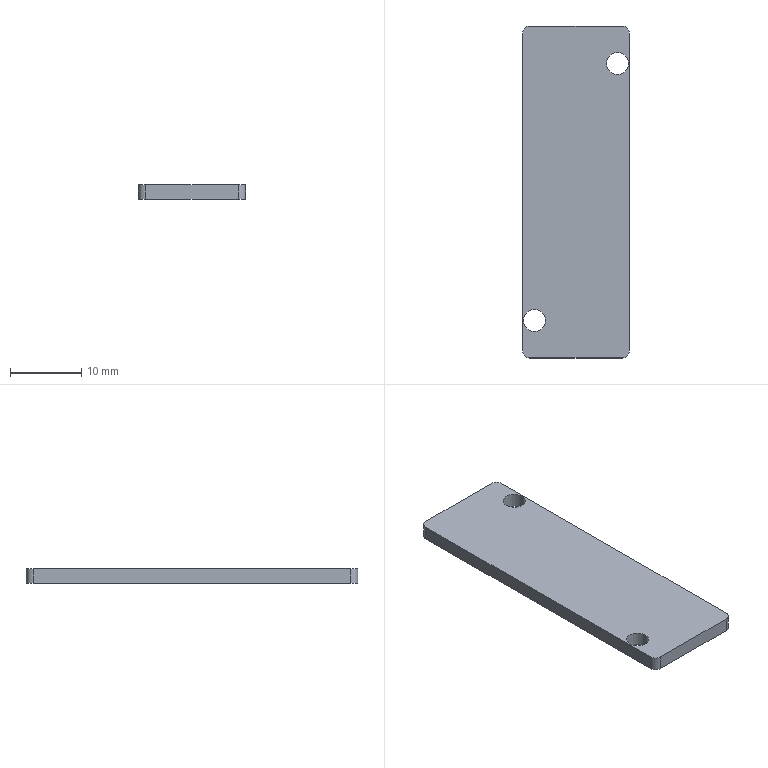Part | STEP file | Blind plate 7V100M | 1 solid | 14 faces | box 15 x 46.5 x 2 mm | volume 1363 mm3 | cylinder 8 | plane 6 | commonest cylinder face diameters 2 x4 3.1 x4
STEP:
#1=CARTESIAN_POINT('',(0.,0.,0.));
#2=DIRECTION('',(0.,0.,1.));
#3=DIRECTION('',(1.,0.,0.));
#4=AXIS2_PLACEMENT_3D('',#1,#2,#3);
#5=CARTESIAN_POINT('',(7.35,18.,0.));
#6=VERTEX_POINT('',#5);
#7=CARTESIAN_POINT('',(7.35,18.,2.));
#8=VERTEX_POINT('',#7);
#9=CARTESIAN_POINT('',(7.35,18.,0.));
#10=DIRECTION('',(0.,0.,1.));
#11=VECTOR('',#10,1.);
#12=LINE('',#9,#11);
#13=CARTESIAN_POINT('',(5.8,18.,0.));
#14=DIRECTION('',(0.,0.,1.));
#15=DIRECTION('',(1.,0.,0.));
#16=AXIS2_PLACEMENT_3D('',#13,#14,#15);
#17=CYLINDRICAL_SURFACE('',#16,1.55);
#18=CARTESIAN_POINT('',(6.283,0.));
#19=DIRECTION('',(0.,1.));
#20=VECTOR('',#19,1.);
#21=LINE('',#18,#20);
#22=(GEOMETRIC_REPRESENTATION_CONTEXT(2)PARAMETRIC_REPRESENTATION_CONTEXT()REPRESENTATION_CONTEXT('',''));
#23=DEFINITIONAL_REPRESENTATION('',(#21),#22);
#24=PCURVE('',#17,#23);
#25=CARTESIAN_POINT('',(5.8,18.,0.));
#26=DIRECTION('',(0.,0.,1.));
#27=DIRECTION('',(1.,0.,0.));
#28=AXIS2_PLACEMENT_3D('',#25,#26,#27);
#29=CYLINDRICAL_SURFACE('',#28,1.55);
#30=CARTESIAN_POINT('',(0.,0.));
#31=DIRECTION('',(0.,1.));
#32=VECTOR('',#31,1.);
#33=LINE('',#30,#32);
#34=(GEOMETRIC_REPRESENTATION_CONTEXT(2)PARAMETRIC_REPRESENTATION_CONTEXT()REPRESENTATION_CONTEXT('',''));
#35=DEFINITIONAL_REPRESENTATION('',(#33),#34);
#36=PCURVE('',#29,#35);
#37=SURFACE_CURVE('',#12,(#24,#36),.PCURVE_S1.);
#38=EDGE_CURVE('',#6,#8,#37,.T.);
#39=ORIENTED_EDGE('',*,*,#38,.T.);
#40=CARTESIAN_POINT('',(4.25,18.,2.));
#41=VERTEX_POINT('',#40);
#42=CARTESIAN_POINT('',(5.8,18.,2.));
#43=DIRECTION('',(0.,0.,1.));
#44=DIRECTION('',(1.,0.,0.));
#45=AXIS2_PLACEMENT_3D('',#42,#43,#44);
#46=CIRCLE('',#45,1.55);
#47=CARTESIAN_POINT('',(0.,2.));
#48=DIRECTION('',(1.,0.));
#49=VECTOR('',#48,1.);
#50=LINE('',#47,#49);
#51=(GEOMETRIC_REPRESENTATION_CONTEXT(2)PARAMETRIC_REPRESENTATION_CONTEXT()REPRESENTATION_CONTEXT('',''));
#52=DEFINITIONAL_REPRESENTATION('',(#50),#51);
#53=PCURVE('',#17,#52);
#54=CARTESIAN_POINT('',(0.,0.,2.));
#55=DIRECTION('',(0.,0.,1.));
#56=DIRECTION('',(1.,0.,0.));
#57=AXIS2_PLACEMENT_3D('',#54,#55,#56);
#58=PLANE('',#57);
#59=CARTESIAN_POINT('',(5.8,18.));
#60=DIRECTION('',(1.,0.));
#61=AXIS2_PLACEMENT_2D('',#59,#60);
#62=CIRCLE('',#61,1.55);
#63=(GEOMETRIC_REPRESENTATION_CONTEXT(2)PARAMETRIC_REPRESENTATION_CONTEXT()REPRESENTATION_CONTEXT('',''));
#64=DEFINITIONAL_REPRESENTATION('',(#62),#63);
#65=PCURVE('',#58,#64);
#66=SURFACE_CURVE('',#46,(#53,#65),.PCURVE_S1.);
#67=EDGE_CURVE('',#41,#8,#66,.T.);
#68=ORIENTED_EDGE('',*,*,#67,.F.);
#69=CARTESIAN_POINT('',(4.25,18.,0.));
#70=VERTEX_POINT('',#69);
#71=CARTESIAN_POINT('',(4.25,18.,0.));
#72=DIRECTION('',(0.,0.,1.));
#73=VECTOR('',#72,1.);
#74=LINE('',#71,#73);
#75=CARTESIAN_POINT('',(3.142,0.));
#76=DIRECTION('',(0.,1.));
#77=VECTOR('',#76,1.);
#78=LINE('',#75,#77);
#79=(GEOMETRIC_REPRESENTATION_CONTEXT(2)PARAMETRIC_REPRESENTATION_CONTEXT()REPRESENTATION_CONTEXT('',''));
#80=DEFINITIONAL_REPRESENTATION('',(#78),#79);
#81=PCURVE('',#17,#80);
#82=CARTESIAN_POINT('',(3.142,0.));
#83=DIRECTION('',(0.,1.));
#84=VECTOR('',#83,1.);
#85=LINE('',#82,#84);
#86=(GEOMETRIC_REPRESENTATION_CONTEXT(2)PARAMETRIC_REPRESENTATION_CONTEXT()REPRESENTATION_CONTEXT('',''));
#87=DEFINITIONAL_REPRESENTATION('',(#85),#86);
#88=PCURVE('',#29,#87);
#89=SURFACE_CURVE('',#74,(#81,#88),.PCURVE_S1.);
#90=EDGE_CURVE('',#70,#41,#89,.T.);
#91=ORIENTED_EDGE('',*,*,#90,.F.);
#92=CARTESIAN_POINT('',(5.8,18.,0.));
#93=DIRECTION('',(0.,0.,1.));
#94=DIRECTION('',(1.,0.,0.));
#95=AXIS2_PLACEMENT_3D('',#92,#93,#94);
#96=CIRCLE('',#95,1.55);
#97=CARTESIAN_POINT('',(0.,0.));
#98=DIRECTION('',(1.,0.));
#99=VECTOR('',#98,1.);
#100=LINE('',#97,#99);
#101=(GEOMETRIC_REPRESENTATION_CONTEXT(2)PARAMETRIC_REPRESENTATION_CONTEXT()REPRESENTATION_CONTEXT('',''));
#102=DEFINITIONAL_REPRESENTATION('',(#100),#101);
#103=PCURVE('',#17,#102);
#104=CARTESIAN_POINT('',(0.,0.,0.));
#105=DIRECTION('',(0.,0.,1.));
#106=DIRECTION('',(1.,0.,0.));
#107=AXIS2_PLACEMENT_3D('',#104,#105,#106);
#108=PLANE('',#107);
#109=CARTESIAN_POINT('',(5.8,18.));
#110=DIRECTION('',(1.,0.));
#111=AXIS2_PLACEMENT_2D('',#109,#110);
#112=CIRCLE('',#111,1.55);
#113=(GEOMETRIC_REPRESENTATION_CONTEXT(2)PARAMETRIC_REPRESENTATION_CONTEXT()REPRESENTATION_CONTEXT('',''));
#114=DEFINITIONAL_REPRESENTATION('',(#112),#113);
#115=PCURVE('',#108,#114);
#116=SURFACE_CURVE('',#96,(#103,#115),.PCURVE_S1.);
#117=EDGE_CURVE('',#70,#6,#116,.T.);
#118=ORIENTED_EDGE('',*,*,#117,.T.);
#119=EDGE_LOOP('',(#39,#68,#91,#118));
#120=FACE_BOUND('',#119,.F.);
#121=ADVANCED_FACE('',(#120),#17,.F.);
#122=CARTESIAN_POINT('',(-4.25,-18.,0.));
#123=VERTEX_POINT('',#122);
#124=CARTESIAN_POINT('',(-4.25,-18.,2.));
#125=VERTEX_POINT('',#124);
#126=CARTESIAN_POINT('',(-4.25,-18.,0.));
#127=DIRECTION('',(0.,0.,1.));
#128=VECTOR('',#127,1.);
#129=LINE('',#126,#128);
#130=CARTESIAN_POINT('',(-5.8,-18.,0.));
#131=DIRECTION('',(0.,0.,1.));
#132=DIRECTION('',(1.,0.,0.));
#133=AXIS2_PLACEMENT_3D('',#130,#131,#132);
#134=CYLINDRICAL_SURFACE('',#133,1.55);
#135=CARTESIAN_POINT('',(6.283,0.));
#136=DIRECTION('',(0.,1.));
#137=VECTOR('',#136,1.);
#138=LINE('',#135,#137);
#139=(GEOMETRIC_REPRESENTATION_CONTEXT(2)PARAMETRIC_REPRESENTATION_CONTEXT()REPRESENTATION_CONTEXT('',''));
#140=DEFINITIONAL_REPRESENTATION('',(#138),#139);
#141=PCURVE('',#134,#140);
#142=CARTESIAN_POINT('',(-5.8,-18.,0.));
#143=DIRECTION('',(0.,0.,1.));
#144=DIRECTION('',(1.,0.,0.));
#145=AXIS2_PLACEMENT_3D('',#142,#143,#144);
#146=CYLINDRICAL_SURFACE('',#145,1.55);
#147=CARTESIAN_POINT('',(0.,0.));
#148=DIRECTION('',(0.,1.));
#149=VECTOR('',#148,1.);
#150=LINE('',#147,#149);
#151=(GEOMETRIC_REPRESENTATION_CONTEXT(2)PARAMETRIC_REPRESENTATION_CONTEXT()REPRESENTATION_CONTEXT('',''));
#152=DEFINITIONAL_REPRESENTATION('',(#150),#151);
#153=PCURVE('',#146,#152);
#154=SURFACE_CURVE('',#129,(#141,#153),.PCURVE_S1.);
#155=EDGE_CURVE('',#123,#125,#154,.T.);
#156=ORIENTED_EDGE('',*,*,#155,.T.);
#157=CARTESIAN_POINT('',(-7.35,-18.,2.));
#158=VERTEX_POINT('',#157);
#159=CARTESIAN_POINT('',(-5.8,-18.,2.));
#160=DIRECTION('',(0.,0.,1.));
#161=DIRECTION('',(1.,0.,0.));
#162=AXIS2_PLACEMENT_3D('',#159,#160,#161);
#163=CIRCLE('',#162,1.55);
#164=CARTESIAN_POINT('',(0.,2.));
#165=DIRECTION('',(1.,0.));
#166=VECTOR('',#165,1.);
#167=LINE('',#164,#166);
#168=(GEOMETRIC_REPRESENTATION_CONTEXT(2)PARAMETRIC_REPRESENTATION_CONTEXT()REPRESENTATION_CONTEXT('',''));
#169=DEFINITIONAL_REPRESENTATION('',(#167),#168);
#170=PCURVE('',#134,#169);
#171=CARTESIAN_POINT('',(-5.8,-18.));
#172=DIRECTION('',(1.,0.));
#173=AXIS2_PLACEMENT_2D('',#171,#172);
#174=CIRCLE('',#173,1.55);
#175=(GEOMETRIC_REPRESENTATION_CONTEXT(2)PARAMETRIC_REPRESENTATION_CONTEXT()REPRESENTATION_CONTEXT('',''));
#176=DEFINITIONAL_REPRESENTATION('',(#174),#175);
#177=PCURVE('',#58,#176);
#178=SURFACE_CURVE('',#163,(#170,#177),.PCURVE_S1.);
#179=EDGE_CURVE('',#158,#125,#178,.T.);
#180=ORIENTED_EDGE('',*,*,#179,.F.);
#181=CARTESIAN_POINT('',(-7.35,-18.,0.));
#182=VERTEX_POINT('',#181);
#183=CARTESIAN_POINT('',(-7.35,-18.,0.));
#184=DIRECTION('',(0.,0.,1.));
#185=VECTOR('',#184,1.);
#186=LINE('',#183,#185);
#187=CARTESIAN_POINT('',(3.142,0.));
#188=DIRECTION('',(0.,1.));
#189=VECTOR('',#188,1.);
#190=LINE('',#187,#189);
#191=(GEOMETRIC_REPRESENTATION_CONTEXT(2)PARAMETRIC_REPRESENTATION_CONTEXT()REPRESENTATION_CONTEXT('',''));
#192=DEFINITIONAL_REPRESENTATION('',(#190),#191);
#193=PCURVE('',#134,#192);
#194=CARTESIAN_POINT('',(3.142,0.));
#195=DIRECTION('',(0.,1.));
#196=VECTOR('',#195,1.);
#197=LINE('',#194,#196);
#198=(GEOMETRIC_REPRESENTATION_CONTEXT(2)PARAMETRIC_REPRESENTATION_CONTEXT()REPRESENTATION_CONTEXT('',''));
#199=DEFINITIONAL_REPRESENTATION('',(#197),#198);
#200=PCURVE('',#146,#199);
#201=SURFACE_CURVE('',#186,(#193,#200),.PCURVE_S1.);
#202=EDGE_CURVE('',#182,#158,#201,.T.);
#203=ORIENTED_EDGE('',*,*,#202,.F.);
#204=CARTESIAN_POINT('',(-5.8,-18.,0.));
#205=DIRECTION('',(0.,0.,1.));
#206=DIRECTION('',(1.,0.,0.));
#207=AXIS2_PLACEMENT_3D('',#204,#205,#206);
#208=CIRCLE('',#207,1.55);
#209=CARTESIAN_POINT('',(0.,0.));
#210=DIRECTION('',(1.,0.));
#211=VECTOR('',#210,1.);
#212=LINE('',#209,#211);
#213=(GEOMETRIC_REPRESENTATION_CONTEXT(2)PARAMETRIC_REPRESENTATION_CONTEXT()REPRESENTATION_CONTEXT('',''));
#214=DEFINITIONAL_REPRESENTATION('',(#212),#213);
#215=PCURVE('',#134,#214);
#216=CARTESIAN_POINT('',(-5.8,-18.));
#217=DIRECTION('',(1.,0.));
#218=AXIS2_PLACEMENT_2D('',#216,#217);
#219=CIRCLE('',#218,1.55);
#220=(GEOMETRIC_REPRESENTATION_CONTEXT(2)PARAMETRIC_REPRESENTATION_CONTEXT()REPRESENTATION_CONTEXT('',''));
#221=DEFINITIONAL_REPRESENTATION('',(#219),#220);
#222=PCURVE('',#108,#221);
#223=SURFACE_CURVE('',#208,(#215,#222),.PCURVE_S1.);
#224=EDGE_CURVE('',#182,#123,#223,.T.);
#225=ORIENTED_EDGE('',*,*,#224,.T.);
#226=EDGE_LOOP('',(#156,#180,#203,#225));
#227=FACE_BOUND('',#226,.F.);
#228=ADVANCED_FACE('',(#227),#134,.F.);
#229=CARTESIAN_POINT('',(-7.5,22.25,0.));
#230=VERTEX_POINT('',#229);
#231=CARTESIAN_POINT('',(-7.5,-22.25,0.));
#232=VERTEX_POINT('',#231);
#233=CARTESIAN_POINT('',(-7.5,-23.25,0.));
#234=DIRECTION('',(0.,-1.,0.));
#235=VECTOR('',#234,1.);
#236=LINE('',#233,#235);
#237=CARTESIAN_POINT('',(-7.5,-23.25,2.));
#238=DIRECTION('',(1.,0.,0.));
#239=DIRECTION('',(0.,0.,-1.));
#240=AXIS2_PLACEMENT_3D('',#237,#238,#239);
#241=PLANE('',#240);
#242=CARTESIAN_POINT('',(2.,0.));
#243=DIRECTION('',(0.,-1.));
#244=VECTOR('',#243,1.);
#245=LINE('',#242,#244);
#246=(GEOMETRIC_REPRESENTATION_CONTEXT(2)PARAMETRIC_REPRESENTATION_CONTEXT()REPRESENTATION_CONTEXT('',''));
#247=DEFINITIONAL_REPRESENTATION('',(#245),#246);
#248=PCURVE('',#241,#247);
#249=CARTESIAN_POINT('',(-7.5,-23.25));
#250=DIRECTION('',(0.,-1.));
#251=VECTOR('',#250,1.);
#252=LINE('',#249,#251);
#253=(GEOMETRIC_REPRESENTATION_CONTEXT(2)PARAMETRIC_REPRESENTATION_CONTEXT()REPRESENTATION_CONTEXT('',''));
#254=DEFINITIONAL_REPRESENTATION('',(#252),#253);
#255=PCURVE('',#108,#254);
#256=SURFACE_CURVE('',#236,(#248,#255),.PCURVE_S1.);
#257=EDGE_CURVE('',#230,#232,#256,.T.);
#258=ORIENTED_EDGE('',*,*,#257,.T.);
#259=CARTESIAN_POINT('',(-7.5,-22.25,2.));
#260=VERTEX_POINT('',#259);
#261=CARTESIAN_POINT('',(-7.5,-22.25,2.));
#262=DIRECTION('',(0.,0.,1.));
#263=VECTOR('',#262,1.);
#264=LINE('',#261,#263);
#265=CARTESIAN_POINT('',(0.,1.));
#266=DIRECTION('',(-1.,0.));
#267=VECTOR('',#266,1.);
#268=LINE('',#265,#267);
#269=(GEOMETRIC_REPRESENTATION_CONTEXT(2)PARAMETRIC_REPRESENTATION_CONTEXT()REPRESENTATION_CONTEXT('',''));
#270=DEFINITIONAL_REPRESENTATION('',(#268),#269);
#271=PCURVE('',#241,#270);
#272=CARTESIAN_POINT('',(-6.5,-22.25,2.));
#273=DIRECTION('',(0.,0.,-1.));
#274=DIRECTION('',(-1.,0.,0.));
#275=AXIS2_PLACEMENT_3D('',#272,#273,#274);
#276=CYLINDRICAL_SURFACE('',#275,1.);
#277=CARTESIAN_POINT('',(6.283,0.));
#278=DIRECTION('',(0.,-1.));
#279=VECTOR('',#278,1.);
#280=LINE('',#277,#279);
#281=(GEOMETRIC_REPRESENTATION_CONTEXT(2)PARAMETRIC_REPRESENTATION_CONTEXT()REPRESENTATION_CONTEXT('',''));
#282=DEFINITIONAL_REPRESENTATION('',(#280),#281);
#283=PCURVE('',#276,#282);
#284=SURFACE_CURVE('',#264,(#271,#283),.PCURVE_S1.);
#285=EDGE_CURVE('',#232,#260,#284,.T.);
#286=ORIENTED_EDGE('',*,*,#285,.T.);
#287=CARTESIAN_POINT('',(-7.5,22.25,2.));
#288=VERTEX_POINT('',#287);
#289=CARTESIAN_POINT('',(-7.5,-23.25,2.));
#290=DIRECTION('',(0.,-1.,0.));
#291=VECTOR('',#290,1.);
#292=LINE('',#289,#291);
#293=CARTESIAN_POINT('',(0.,0.));
#294=DIRECTION('',(0.,-1.));
#295=VECTOR('',#294,1.);
#296=LINE('',#293,#295);
#297=(GEOMETRIC_REPRESENTATION_CONTEXT(2)PARAMETRIC_REPRESENTATION_CONTEXT()REPRESENTATION_CONTEXT('',''));
#298=DEFINITIONAL_REPRESENTATION('',(#296),#297);
#299=PCURVE('',#241,#298);
#300=CARTESIAN_POINT('',(-7.5,-23.25));
#301=DIRECTION('',(0.,-1.));
#302=VECTOR('',#301,1.);
#303=LINE('',#300,#302);
#304=(GEOMETRIC_REPRESENTATION_CONTEXT(2)PARAMETRIC_REPRESENTATION_CONTEXT()REPRESENTATION_CONTEXT('',''));
#305=DEFINITIONAL_REPRESENTATION('',(#303),#304);
#306=PCURVE('',#58,#305);
#307=SURFACE_CURVE('',#292,(#299,#306),.PCURVE_S1.);
#308=EDGE_CURVE('',#288,#260,#307,.T.);
#309=ORIENTED_EDGE('',*,*,#308,.F.);
#310=CARTESIAN_POINT('',(-7.5,22.25,2.));
#311=DIRECTION('',(0.,0.,-1.));
#312=VECTOR('',#311,1.);
#313=LINE('',#310,#312);
#314=CARTESIAN_POINT('',(0.,45.5));
#315=DIRECTION('',(1.,0.));
#316=VECTOR('',#315,1.);
#317=LINE('',#314,#316);
#318=(GEOMETRIC_REPRESENTATION_CONTEXT(2)PARAMETRIC_REPRESENTATION_CONTEXT()REPRESENTATION_CONTEXT('',''));
#319=DEFINITIONAL_REPRESENTATION('',(#317),#318);
#320=PCURVE('',#241,#319);
#321=CARTESIAN_POINT('',(-6.5,22.25,2.));
#322=DIRECTION('',(0.,0.,-1.));
#323=DIRECTION('',(-1.,0.,0.));
#324=AXIS2_PLACEMENT_3D('',#321,#322,#323);
#325=CYLINDRICAL_SURFACE('',#324,1.);
#326=CARTESIAN_POINT('',(0.,0.));
#327=DIRECTION('',(0.,1.));
#328=VECTOR('',#327,1.);
#329=LINE('',#326,#328);
#330=(GEOMETRIC_REPRESENTATION_CONTEXT(2)PARAMETRIC_REPRESENTATION_CONTEXT()REPRESENTATION_CONTEXT('',''));
#331=DEFINITIONAL_REPRESENTATION('',(#329),#330);
#332=PCURVE('',#325,#331);
#333=SURFACE_CURVE('',#313,(#320,#332),.PCURVE_S1.);
#334=EDGE_CURVE('',#288,#230,#333,.T.);
#335=ORIENTED_EDGE('',*,*,#334,.T.);
#336=EDGE_LOOP('',(#258,#286,#309,#335));
#337=FACE_BOUND('',#336,.T.);
#338=ADVANCED_FACE('',(#337),#241,.F.);
#339=CARTESIAN_POINT('',(-6.5,-23.25,0.));
#340=VERTEX_POINT('',#339);
#341=CARTESIAN_POINT('',(6.5,-23.25,0.));
#342=VERTEX_POINT('',#341);
#343=CARTESIAN_POINT('',(7.5,-23.25,0.));
#344=DIRECTION('',(1.,0.,0.));
#345=VECTOR('',#344,1.);
#346=LINE('',#343,#345);
#347=CARTESIAN_POINT('',(7.5,-23.25,2.));
#348=DIRECTION('',(0.,1.,0.));
#349=DIRECTION('',(-1.,0.,0.));
#350=AXIS2_PLACEMENT_3D('',#347,#348,#349);
#351=PLANE('',#350);
#352=CARTESIAN_POINT('',(0.,-2.));
#353=DIRECTION('',(-1.,0.));
#354=VECTOR('',#353,1.);
#355=LINE('',#352,#354);
#356=(GEOMETRIC_REPRESENTATION_CONTEXT(2)PARAMETRIC_REPRESENTATION_CONTEXT()REPRESENTATION_CONTEXT('',''));
#357=DEFINITIONAL_REPRESENTATION('',(#355),#356);
#358=PCURVE('',#351,#357);
#359=CARTESIAN_POINT('',(7.5,-23.25));
#360=DIRECTION('',(1.,0.));
#361=VECTOR('',#360,1.);
#362=LINE('',#359,#361);
#363=(GEOMETRIC_REPRESENTATION_CONTEXT(2)PARAMETRIC_REPRESENTATION_CONTEXT()REPRESENTATION_CONTEXT('',''));
#364=DEFINITIONAL_REPRESENTATION('',(#362),#363);
#365=PCURVE('',#108,#364);
#366=SURFACE_CURVE('',#346,(#358,#365),.PCURVE_S1.);
#367=EDGE_CURVE('',#340,#342,#366,.T.);
#368=ORIENTED_EDGE('',*,*,#367,.T.);
#369=CARTESIAN_POINT('',(6.5,-23.25,2.));
#370=VERTEX_POINT('',#369);
#371=CARTESIAN_POINT('',(6.5,-23.25,2.));
#372=DIRECTION('',(0.,0.,1.));
#373=VECTOR('',#372,1.);
#374=LINE('',#371,#373);
#375=CARTESIAN_POINT('',(1.,0.));
#376=DIRECTION('',(0.,1.));
#377=VECTOR('',#376,1.);
#378=LINE('',#375,#377);
#379=(GEOMETRIC_REPRESENTATION_CONTEXT(2)PARAMETRIC_REPRESENTATION_CONTEXT()REPRESENTATION_CONTEXT('',''));
#380=DEFINITIONAL_REPRESENTATION('',(#378),#379);
#381=PCURVE('',#351,#380);
#382=CARTESIAN_POINT('',(6.5,-22.25,2.));
#383=DIRECTION('',(0.,0.,-1.));
#384=DIRECTION('',(-1.,0.,0.));
#385=AXIS2_PLACEMENT_3D('',#382,#383,#384);
#386=CYLINDRICAL_SURFACE('',#385,1.);
#387=CARTESIAN_POINT('',(4.712,0.));
#388=DIRECTION('',(0.,-1.));
#389=VECTOR('',#388,1.);
#390=LINE('',#387,#389);
#391=(GEOMETRIC_REPRESENTATION_CONTEXT(2)PARAMETRIC_REPRESENTATION_CONTEXT()REPRESENTATION_CONTEXT('',''));
#392=DEFINITIONAL_REPRESENTATION('',(#390),#391);
#393=PCURVE('',#386,#392);
#394=SURFACE_CURVE('',#374,(#381,#393),.PCURVE_S1.);
#395=EDGE_CURVE('',#342,#370,#394,.T.);
#396=ORIENTED_EDGE('',*,*,#395,.T.);
#397=CARTESIAN_POINT('',(-6.5,-23.25,2.));
#398=VERTEX_POINT('',#397);
#399=CARTESIAN_POINT('',(7.5,-23.25,2.));
#400=DIRECTION('',(1.,0.,0.));
#401=VECTOR('',#400,1.);
#402=LINE('',#399,#401);
#403=CARTESIAN_POINT('',(0.,0.));
#404=DIRECTION('',(-1.,0.));
#405=VECTOR('',#404,1.);
#406=LINE('',#403,#405);
#407=(GEOMETRIC_REPRESENTATION_CONTEXT(2)PARAMETRIC_REPRESENTATION_CONTEXT()REPRESENTATION_CONTEXT('',''));
#408=DEFINITIONAL_REPRESENTATION('',(#406),#407);
#409=PCURVE('',#351,#408);
#410=CARTESIAN_POINT('',(7.5,-23.25));
#411=DIRECTION('',(1.,0.));
#412=VECTOR('',#411,1.);
#413=LINE('',#410,#412);
#414=(GEOMETRIC_REPRESENTATION_CONTEXT(2)PARAMETRIC_REPRESENTATION_CONTEXT()REPRESENTATION_CONTEXT('',''));
#415=DEFINITIONAL_REPRESENTATION('',(#413),#414);
#416=PCURVE('',#58,#415);
#417=SURFACE_CURVE('',#402,(#409,#416),.PCURVE_S1.);
#418=EDGE_CURVE('',#398,#370,#417,.T.);
#419=ORIENTED_EDGE('',*,*,#418,.F.);
#420=CARTESIAN_POINT('',(-6.5,-23.25,2.));
#421=DIRECTION('',(0.,0.,-1.));
#422=VECTOR('',#421,1.);
#423=LINE('',#420,#422);
#424=CARTESIAN_POINT('',(14.,0.));
#425=DIRECTION('',(0.,-1.));
#426=VECTOR('',#425,1.);
#427=LINE('',#424,#426);
#428=(GEOMETRIC_REPRESENTATION_CONTEXT(2)PARAMETRIC_REPRESENTATION_CONTEXT()REPRESENTATION_CONTEXT('',''));
#429=DEFINITIONAL_REPRESENTATION('',(#427),#428);
#430=PCURVE('',#351,#429);
#431=CARTESIAN_POINT('',(4.712,0.));
#432=DIRECTION('',(0.,1.));
#433=VECTOR('',#432,1.);
#434=LINE('',#431,#433);
#435=(GEOMETRIC_REPRESENTATION_CONTEXT(2)PARAMETRIC_REPRESENTATION_CONTEXT()REPRESENTATION_CONTEXT('',''));
#436=DEFINITIONAL_REPRESENTATION('',(#434),#435);
#437=PCURVE('',#276,#436);
#438=SURFACE_CURVE('',#423,(#430,#437),.PCURVE_S1.);
#439=EDGE_CURVE('',#398,#340,#438,.T.);
#440=ORIENTED_EDGE('',*,*,#439,.T.);
#441=EDGE_LOOP('',(#368,#396,#419,#440));
#442=FACE_BOUND('',#441,.T.);
#443=ADVANCED_FACE('',(#442),#351,.F.);
#444=CARTESIAN_POINT('',(7.5,-22.25,2.));
#445=VERTEX_POINT('',#444);
#446=CARTESIAN_POINT('',(7.5,22.25,2.));
#447=VERTEX_POINT('',#446);
#448=CARTESIAN_POINT('',(7.5,-23.25,2.));
#449=DIRECTION('',(0.,1.,0.));
#450=VECTOR('',#449,1.);
#451=LINE('',#448,#450);
#452=CARTESIAN_POINT('',(7.5,-23.25,2.));
#453=DIRECTION('',(-1.,0.,0.));
#454=DIRECTION('',(0.,0.,1.));
#455=AXIS2_PLACEMENT_3D('',#452,#453,#454);
#456=PLANE('',#455);
#457=CARTESIAN_POINT('',(0.,0.));
#458=DIRECTION('',(0.,1.));
#459=VECTOR('',#458,1.);
#460=LINE('',#457,#459);
#461=(GEOMETRIC_REPRESENTATION_CONTEXT(2)PARAMETRIC_REPRESENTATION_CONTEXT()REPRESENTATION_CONTEXT('',''));
#462=DEFINITIONAL_REPRESENTATION('',(#460),#461);
#463=PCURVE('',#456,#462);
#464=CARTESIAN_POINT('',(7.5,-23.25));
#465=DIRECTION('',(0.,1.));
#466=VECTOR('',#465,1.);
#467=LINE('',#464,#466);
#468=(GEOMETRIC_REPRESENTATION_CONTEXT(2)PARAMETRIC_REPRESENTATION_CONTEXT()REPRESENTATION_CONTEXT('',''));
#469=DEFINITIONAL_REPRESENTATION('',(#467),#468);
#470=PCURVE('',#58,#469);
#471=SURFACE_CURVE('',#451,(#463,#470),.PCURVE_S1.);
#472=EDGE_CURVE('',#445,#447,#471,.T.);
#473=ORIENTED_EDGE('',*,*,#472,.F.);
#474=CARTESIAN_POINT('',(7.5,-22.25,0.));
#475=VERTEX_POINT('',#474);
#476=CARTESIAN_POINT('',(7.5,-22.25,2.));
#477=DIRECTION('',(0.,0.,-1.));
#478=VECTOR('',#477,1.);
#479=LINE('',#476,#478);
#480=CARTESIAN_POINT('',(0.,1.));
#481=DIRECTION('',(-1.,0.));
#482=VECTOR('',#481,1.);
#483=LINE('',#480,#482);
#484=(GEOMETRIC_REPRESENTATION_CONTEXT(2)PARAMETRIC_REPRESENTATION_CONTEXT()REPRESENTATION_CONTEXT('',''));
#485=DEFINITIONAL_REPRESENTATION('',(#483),#484);
#486=PCURVE('',#456,#485);
#487=CARTESIAN_POINT('',(3.142,0.));
#488=DIRECTION('',(0.,1.));
#489=VECTOR('',#488,1.);
#490=LINE('',#487,#489);
#491=(GEOMETRIC_REPRESENTATION_CONTEXT(2)PARAMETRIC_REPRESENTATION_CONTEXT()REPRESENTATION_CONTEXT('',''));
#492=DEFINITIONAL_REPRESENTATION('',(#490),#491);
#493=PCURVE('',#386,#492);
#494=SURFACE_CURVE('',#479,(#486,#493),.PCURVE_S1.);
#495=EDGE_CURVE('',#445,#475,#494,.T.);
#496=ORIENTED_EDGE('',*,*,#495,.T.);
#497=CARTESIAN_POINT('',(7.5,22.25,0.));
#498=VERTEX_POINT('',#497);
#499=CARTESIAN_POINT('',(7.5,-23.25,0.));
#500=DIRECTION('',(0.,1.,0.));
#501=VECTOR('',#500,1.);
#502=LINE('',#499,#501);
#503=CARTESIAN_POINT('',(-2.,0.));
#504=DIRECTION('',(0.,1.));
#505=VECTOR('',#504,1.);
#506=LINE('',#503,#505);
#507=(GEOMETRIC_REPRESENTATION_CONTEXT(2)PARAMETRIC_REPRESENTATION_CONTEXT()REPRESENTATION_CONTEXT('',''));
#508=DEFINITIONAL_REPRESENTATION('',(#506),#507);
#509=PCURVE('',#456,#508);
#510=CARTESIAN_POINT('',(7.5,-23.25));
#511=DIRECTION('',(0.,1.));
#512=VECTOR('',#511,1.);
#513=LINE('',#510,#512);
#514=(GEOMETRIC_REPRESENTATION_CONTEXT(2)PARAMETRIC_REPRESENTATION_CONTEXT()REPRESENTATION_CONTEXT('',''));
#515=DEFINITIONAL_REPRESENTATION('',(#513),#514);
#516=PCURVE('',#108,#515);
#517=SURFACE_CURVE('',#502,(#509,#516),.PCURVE_S1.);
#518=EDGE_CURVE('',#475,#498,#517,.T.);
#519=ORIENTED_EDGE('',*,*,#518,.T.);
#520=CARTESIAN_POINT('',(7.5,22.25,2.));
#521=DIRECTION('',(0.,0.,1.));
#522=VECTOR('',#521,1.);
#523=LINE('',#520,#522);
#524=CARTESIAN_POINT('',(0.,45.5));
#525=DIRECTION('',(1.,0.));
#526=VECTOR('',#525,1.);
#527=LINE('',#524,#526);
#528=(GEOMETRIC_REPRESENTATION_CONTEXT(2)PARAMETRIC_REPRESENTATION_CONTEXT()REPRESENTATION_CONTEXT('',''));
#529=DEFINITIONAL_REPRESENTATION('',(#527),#528);
#530=PCURVE('',#456,#529);
#531=CARTESIAN_POINT('',(6.5,22.25,2.));
#532=DIRECTION('',(0.,0.,-1.));
#533=DIRECTION('',(-1.,0.,0.));
#534=AXIS2_PLACEMENT_3D('',#531,#532,#533);
#535=CYLINDRICAL_SURFACE('',#534,1.);
#536=CARTESIAN_POINT('',(3.142,0.));
#537=DIRECTION('',(0.,-1.));
#538=VECTOR('',#537,1.);
#539=LINE('',#536,#538);
#540=(GEOMETRIC_REPRESENTATION_CONTEXT(2)PARAMETRIC_REPRESENTATION_CONTEXT()REPRESENTATION_CONTEXT('',''));
#541=DEFINITIONAL_REPRESENTATION('',(#539),#540);
#542=PCURVE('',#535,#541);
#543=SURFACE_CURVE('',#523,(#530,#542),.PCURVE_S1.);
#544=EDGE_CURVE('',#498,#447,#543,.T.);
#545=ORIENTED_EDGE('',*,*,#544,.T.);
#546=EDGE_LOOP('',(#473,#496,#519,#545));
#547=FACE_BOUND('',#546,.T.);
#548=ADVANCED_FACE('',(#547),#456,.F.);
#549=CARTESIAN_POINT('',(6.5,23.25,2.));
#550=VERTEX_POINT('',#549);
#551=CARTESIAN_POINT('',(-6.5,23.25,2.));
#552=VERTEX_POINT('',#551);
#553=CARTESIAN_POINT('',(7.5,23.25,2.));
#554=DIRECTION('',(-1.,0.,0.));
#555=VECTOR('',#554,1.);
#556=LINE('',#553,#555);
#557=CARTESIAN_POINT('',(7.5,23.25,2.));
#558=DIRECTION('',(0.,-1.,0.));
#559=DIRECTION('',(0.,0.,-1.));
#560=AXIS2_PLACEMENT_3D('',#557,#558,#559);
#561=PLANE('',#560);
#562=CARTESIAN_POINT('',(0.,0.));
#563=DIRECTION('',(0.,-1.));
#564=VECTOR('',#563,1.);
#565=LINE('',#562,#564);
#566=(GEOMETRIC_REPRESENTATION_CONTEXT(2)PARAMETRIC_REPRESENTATION_CONTEXT()REPRESENTATION_CONTEXT('',''));
#567=DEFINITIONAL_REPRESENTATION('',(#565),#566);
#568=PCURVE('',#561,#567);
#569=CARTESIAN_POINT('',(7.5,23.25));
#570=DIRECTION('',(-1.,0.));
#571=VECTOR('',#570,1.);
#572=LINE('',#569,#571);
#573=(GEOMETRIC_REPRESENTATION_CONTEXT(2)PARAMETRIC_REPRESENTATION_CONTEXT()REPRESENTATION_CONTEXT('',''));
#574=DEFINITIONAL_REPRESENTATION('',(#572),#573);
#575=PCURVE('',#58,#574);
#576=SURFACE_CURVE('',#556,(#568,#575),.PCURVE_S1.);
#577=EDGE_CURVE('',#550,#552,#576,.T.);
#578=ORIENTED_EDGE('',*,*,#577,.F.);
#579=CARTESIAN_POINT('',(6.5,23.25,0.));
#580=VERTEX_POINT('',#579);
#581=CARTESIAN_POINT('',(6.5,23.25,2.));
#582=DIRECTION('',(0.,0.,-1.));
#583=VECTOR('',#582,1.);
#584=LINE('',#581,#583);
#585=CARTESIAN_POINT('',(0.,-1.));
#586=DIRECTION('',(1.,0.));
#587=VECTOR('',#586,1.);
#588=LINE('',#585,#587);
#589=(GEOMETRIC_REPRESENTATION_CONTEXT(2)PARAMETRIC_REPRESENTATION_CONTEXT()REPRESENTATION_CONTEXT('',''));
#590=DEFINITIONAL_REPRESENTATION('',(#588),#589);
#591=PCURVE('',#561,#590);
#592=CARTESIAN_POINT('',(1.571,0.));
#593=DIRECTION('',(0.,1.));
#594=VECTOR('',#593,1.);
#595=LINE('',#592,#594);
#596=(GEOMETRIC_REPRESENTATION_CONTEXT(2)PARAMETRIC_REPRESENTATION_CONTEXT()REPRESENTATION_CONTEXT('',''));
#597=DEFINITIONAL_REPRESENTATION('',(#595),#596);
#598=PCURVE('',#535,#597);
#599=SURFACE_CURVE('',#584,(#591,#598),.PCURVE_S1.);
#600=EDGE_CURVE('',#550,#580,#599,.T.);
#601=ORIENTED_EDGE('',*,*,#600,.T.);
#602=CARTESIAN_POINT('',(-6.5,23.25,0.));
#603=VERTEX_POINT('',#602);
#604=CARTESIAN_POINT('',(7.5,23.25,0.));
#605=DIRECTION('',(-1.,0.,0.));
#606=VECTOR('',#605,1.);
#607=LINE('',#604,#606);
#608=CARTESIAN_POINT('',(2.,0.));
#609=DIRECTION('',(0.,-1.));
#610=VECTOR('',#609,1.);
#611=LINE('',#608,#610);
#612=(GEOMETRIC_REPRESENTATION_CONTEXT(2)PARAMETRIC_REPRESENTATION_CONTEXT()REPRESENTATION_CONTEXT('',''));
#613=DEFINITIONAL_REPRESENTATION('',(#611),#612);
#614=PCURVE('',#561,#613);
#615=CARTESIAN_POINT('',(7.5,23.25));
#616=DIRECTION('',(-1.,0.));
#617=VECTOR('',#616,1.);
#618=LINE('',#615,#617);
#619=(GEOMETRIC_REPRESENTATION_CONTEXT(2)PARAMETRIC_REPRESENTATION_CONTEXT()REPRESENTATION_CONTEXT('',''));
#620=DEFINITIONAL_REPRESENTATION('',(#618),#619);
#621=PCURVE('',#108,#620);
#622=SURFACE_CURVE('',#607,(#614,#621),.PCURVE_S1.);
#623=EDGE_CURVE('',#580,#603,#622,.T.);
#624=ORIENTED_EDGE('',*,*,#623,.T.);
#625=CARTESIAN_POINT('',(-6.5,23.25,2.));
#626=DIRECTION('',(0.,0.,1.));
#627=VECTOR('',#626,1.);
#628=LINE('',#625,#627);
#629=CARTESIAN_POINT('',(0.,-14.));
#630=DIRECTION('',(-1.,0.));
#631=VECTOR('',#630,1.);
#632=LINE('',#629,#631);
#633=(GEOMETRIC_REPRESENTATION_CONTEXT(2)PARAMETRIC_REPRESENTATION_CONTEXT()REPRESENTATION_CONTEXT('',''));
#634=DEFINITIONAL_REPRESENTATION('',(#632),#633);
#635=PCURVE('',#561,#634);
#636=CARTESIAN_POINT('',(1.571,0.));
#637=DIRECTION('',(0.,-1.));
#638=VECTOR('',#637,1.);
#639=LINE('',#636,#638);
#640=(GEOMETRIC_REPRESENTATION_CONTEXT(2)PARAMETRIC_REPRESENTATION_CONTEXT()REPRESENTATION_CONTEXT('',''));
#641=DEFINITIONAL_REPRESENTATION('',(#639),#640);
#642=PCURVE('',#325,#641);
#643=SURFACE_CURVE('',#628,(#635,#642),.PCURVE_S1.);
#644=EDGE_CURVE('',#603,#552,#643,.T.);
#645=ORIENTED_EDGE('',*,*,#644,.T.);
#646=EDGE_LOOP('',(#578,#601,#624,#645));
#647=FACE_BOUND('',#646,.T.);
#648=ADVANCED_FACE('',(#647),#561,.F.);
#649=CARTESIAN_POINT('',(5.8,18.,2.));
#650=DIRECTION('',(0.,0.,1.));
#651=DIRECTION('',(1.,0.,0.));
#652=AXIS2_PLACEMENT_3D('',#649,#650,#651);
#653=CIRCLE('',#652,1.55);
#654=CARTESIAN_POINT('',(5.8,18.));
#655=DIRECTION('',(1.,0.));
#656=AXIS2_PLACEMENT_2D('',#654,#655);
#657=CIRCLE('',#656,1.55);
#658=(GEOMETRIC_REPRESENTATION_CONTEXT(2)PARAMETRIC_REPRESENTATION_CONTEXT()REPRESENTATION_CONTEXT('',''));
#659=DEFINITIONAL_REPRESENTATION('',(#657),#658);
#660=PCURVE('',#58,#659);
#661=CARTESIAN_POINT('',(0.,2.));
#662=DIRECTION('',(1.,0.));
#663=VECTOR('',#662,1.);
#664=LINE('',#661,#663);
#665=(GEOMETRIC_REPRESENTATION_CONTEXT(2)PARAMETRIC_REPRESENTATION_CONTEXT()REPRESENTATION_CONTEXT('',''));
#666=DEFINITIONAL_REPRESENTATION('',(#664),#665);
#667=PCURVE('',#29,#666);
#668=SURFACE_CURVE('',#653,(#660,#667),.PCURVE_S1.);
#669=EDGE_CURVE('',#8,#41,#668,.T.);
#670=ORIENTED_EDGE('',*,*,#669,.F.);
#671=ORIENTED_EDGE('',*,*,#67,.F.);
#672=EDGE_LOOP('',(#670,#671));
#673=FACE_BOUND('',#672,.T.);
#674=CARTESIAN_POINT('',(-5.8,-18.,2.));
#675=DIRECTION('',(0.,0.,1.));
#676=DIRECTION('',(1.,0.,0.));
#677=AXIS2_PLACEMENT_3D('',#674,#675,#676);
#678=CIRCLE('',#677,1.55);
#679=CARTESIAN_POINT('',(-5.8,-18.));
#680=DIRECTION('',(1.,0.));
#681=AXIS2_PLACEMENT_2D('',#679,#680);
#682=CIRCLE('',#681,1.55);
#683=(GEOMETRIC_REPRESENTATION_CONTEXT(2)PARAMETRIC_REPRESENTATION_CONTEXT()REPRESENTATION_CONTEXT('',''));
#684=DEFINITIONAL_REPRESENTATION('',(#682),#683);
#685=PCURVE('',#58,#684);
#686=CARTESIAN_POINT('',(0.,2.));
#687=DIRECTION('',(1.,0.));
#688=VECTOR('',#687,1.);
#689=LINE('',#686,#688);
#690=(GEOMETRIC_REPRESENTATION_CONTEXT(2)PARAMETRIC_REPRESENTATION_CONTEXT()REPRESENTATION_CONTEXT('',''));
#691=DEFINITIONAL_REPRESENTATION('',(#689),#690);
#692=PCURVE('',#146,#691);
#693=SURFACE_CURVE('',#678,(#685,#692),.PCURVE_S1.);
#694=EDGE_CURVE('',#125,#158,#693,.T.);
#695=ORIENTED_EDGE('',*,*,#694,.F.);
#696=ORIENTED_EDGE('',*,*,#179,.F.);
#697=EDGE_LOOP('',(#695,#696));
#698=FACE_BOUND('',#697,.T.);
#699=ORIENTED_EDGE('',*,*,#418,.T.);
#700=CARTESIAN_POINT('',(6.5,-22.25,2.));
#701=DIRECTION('',(0.,0.,1.));
#702=DIRECTION('',(1.,0.,0.));
#703=AXIS2_PLACEMENT_3D('',#700,#701,#702);
#704=CIRCLE('',#703,1.);
#705=CARTESIAN_POINT('',(6.5,-22.25));
#706=DIRECTION('',(1.,0.));
#707=AXIS2_PLACEMENT_2D('',#705,#706);
#708=CIRCLE('',#707,1.);
#709=(GEOMETRIC_REPRESENTATION_CONTEXT(2)PARAMETRIC_REPRESENTATION_CONTEXT()REPRESENTATION_CONTEXT('',''));
#710=DEFINITIONAL_REPRESENTATION('',(#708),#709);
#711=PCURVE('',#58,#710);
#712=CARTESIAN_POINT('',(9.425,0.));
#713=DIRECTION('',(-1.,0.));
#714=VECTOR('',#713,1.);
#715=LINE('',#712,#714);
#716=(GEOMETRIC_REPRESENTATION_CONTEXT(2)PARAMETRIC_REPRESENTATION_CONTEXT()REPRESENTATION_CONTEXT('',''));
#717=DEFINITIONAL_REPRESENTATION('',(#715),#716);
#718=PCURVE('',#386,#717);
#719=SURFACE_CURVE('',#704,(#711,#718),.PCURVE_S1.);
#720=EDGE_CURVE('',#370,#445,#719,.T.);
#721=ORIENTED_EDGE('',*,*,#720,.T.);
#722=ORIENTED_EDGE('',*,*,#472,.T.);
#723=CARTESIAN_POINT('',(6.5,22.25,2.));
#724=DIRECTION('',(0.,0.,1.));
#725=DIRECTION('',(1.,0.,0.));
#726=AXIS2_PLACEMENT_3D('',#723,#724,#725);
#727=CIRCLE('',#726,1.);
#728=CARTESIAN_POINT('',(6.5,22.25));
#729=DIRECTION('',(1.,0.));
#730=AXIS2_PLACEMENT_2D('',#728,#729);
#731=CIRCLE('',#730,1.);
#732=(GEOMETRIC_REPRESENTATION_CONTEXT(2)PARAMETRIC_REPRESENTATION_CONTEXT()REPRESENTATION_CONTEXT('',''));
#733=DEFINITIONAL_REPRESENTATION('',(#731),#732);
#734=PCURVE('',#58,#733);
#735=CARTESIAN_POINT('',(3.142,0.));
#736=DIRECTION('',(-1.,0.));
#737=VECTOR('',#736,1.);
#738=LINE('',#735,#737);
#739=(GEOMETRIC_REPRESENTATION_CONTEXT(2)PARAMETRIC_REPRESENTATION_CONTEXT()REPRESENTATION_CONTEXT('',''));
#740=DEFINITIONAL_REPRESENTATION('',(#738),#739);
#741=PCURVE('',#535,#740);
#742=SURFACE_CURVE('',#727,(#734,#741),.PCURVE_S1.);
#743=EDGE_CURVE('',#447,#550,#742,.T.);
#744=ORIENTED_EDGE('',*,*,#743,.T.);
#745=ORIENTED_EDGE('',*,*,#577,.T.);
#746=CARTESIAN_POINT('',(-6.5,22.25,2.));
#747=DIRECTION('',(0.,0.,1.));
#748=DIRECTION('',(1.,0.,0.));
#749=AXIS2_PLACEMENT_3D('',#746,#747,#748);
#750=CIRCLE('',#749,1.);
#751=CARTESIAN_POINT('',(-6.5,22.25));
#752=DIRECTION('',(1.,0.));
#753=AXIS2_PLACEMENT_2D('',#751,#752);
#754=CIRCLE('',#753,1.);
#755=(GEOMETRIC_REPRESENTATION_CONTEXT(2)PARAMETRIC_REPRESENTATION_CONTEXT()REPRESENTATION_CONTEXT('',''));
#756=DEFINITIONAL_REPRESENTATION('',(#754),#755);
#757=PCURVE('',#58,#756);
#758=CARTESIAN_POINT('',(3.142,0.));
#759=DIRECTION('',(-1.,0.));
#760=VECTOR('',#759,1.);
#761=LINE('',#758,#760);
#762=(GEOMETRIC_REPRESENTATION_CONTEXT(2)PARAMETRIC_REPRESENTATION_CONTEXT()REPRESENTATION_CONTEXT('',''));
#763=DEFINITIONAL_REPRESENTATION('',(#761),#762);
#764=PCURVE('',#325,#763);
#765=SURFACE_CURVE('',#750,(#757,#764),.PCURVE_S1.);
#766=EDGE_CURVE('',#552,#288,#765,.T.);
#767=ORIENTED_EDGE('',*,*,#766,.T.);
#768=ORIENTED_EDGE('',*,*,#308,.T.);
#769=CARTESIAN_POINT('',(-6.5,-22.25,2.));
#770=DIRECTION('',(0.,0.,1.));
#771=DIRECTION('',(1.,0.,0.));
#772=AXIS2_PLACEMENT_3D('',#769,#770,#771);
#773=CIRCLE('',#772,1.);
#774=CARTESIAN_POINT('',(-6.5,-22.25));
#775=DIRECTION('',(1.,0.));
#776=AXIS2_PLACEMENT_2D('',#774,#775);
#777=CIRCLE('',#776,1.);
#778=(GEOMETRIC_REPRESENTATION_CONTEXT(2)PARAMETRIC_REPRESENTATION_CONTEXT()REPRESENTATION_CONTEXT('',''));
#779=DEFINITIONAL_REPRESENTATION('',(#777),#778);
#780=PCURVE('',#58,#779);
#781=CARTESIAN_POINT('',(9.425,0.));
#782=DIRECTION('',(-1.,0.));
#783=VECTOR('',#782,1.);
#784=LINE('',#781,#783);
#785=(GEOMETRIC_REPRESENTATION_CONTEXT(2)PARAMETRIC_REPRESENTATION_CONTEXT()REPRESENTATION_CONTEXT('',''));
#786=DEFINITIONAL_REPRESENTATION('',(#784),#785);
#787=PCURVE('',#276,#786);
#788=SURFACE_CURVE('',#773,(#780,#787),.PCURVE_S1.);
#789=EDGE_CURVE('',#260,#398,#788,.T.);
#790=ORIENTED_EDGE('',*,*,#789,.T.);
#791=EDGE_LOOP('',(#699,#721,#722,#744,#745,#767,#768,#790));
#792=FACE_BOUND('',#791,.T.);
#793=ADVANCED_FACE('',(#673,#698,#792),#58,.T.);
#794=CARTESIAN_POINT('',(5.8,18.,0.));
#795=DIRECTION('',(0.,0.,1.));
#796=DIRECTION('',(1.,0.,0.));
#797=AXIS2_PLACEMENT_3D('',#794,#795,#796);
#798=CIRCLE('',#797,1.55);
#799=CARTESIAN_POINT('',(5.8,18.));
#800=DIRECTION('',(1.,0.));
#801=AXIS2_PLACEMENT_2D('',#799,#800);
#802=CIRCLE('',#801,1.55);
#803=(GEOMETRIC_REPRESENTATION_CONTEXT(2)PARAMETRIC_REPRESENTATION_CONTEXT()REPRESENTATION_CONTEXT('',''));
#804=DEFINITIONAL_REPRESENTATION('',(#802),#803);
#805=PCURVE('',#108,#804);
#806=CARTESIAN_POINT('',(0.,0.));
#807=DIRECTION('',(1.,0.));
#808=VECTOR('',#807,1.);
#809=LINE('',#806,#808);
#810=(GEOMETRIC_REPRESENTATION_CONTEXT(2)PARAMETRIC_REPRESENTATION_CONTEXT()REPRESENTATION_CONTEXT('',''));
#811=DEFINITIONAL_REPRESENTATION('',(#809),#810);
#812=PCURVE('',#29,#811);
#813=SURFACE_CURVE('',#798,(#805,#812),.PCURVE_S1.);
#814=EDGE_CURVE('',#6,#70,#813,.T.);
#815=ORIENTED_EDGE('',*,*,#814,.T.);
#816=ORIENTED_EDGE('',*,*,#117,.T.);
#817=EDGE_LOOP('',(#815,#816));
#818=FACE_BOUND('',#817,.T.);
#819=CARTESIAN_POINT('',(-5.8,-18.,0.));
#820=DIRECTION('',(0.,0.,1.));
#821=DIRECTION('',(1.,0.,0.));
#822=AXIS2_PLACEMENT_3D('',#819,#820,#821);
#823=CIRCLE('',#822,1.55);
#824=CARTESIAN_POINT('',(-5.8,-18.));
#825=DIRECTION('',(1.,0.));
#826=AXIS2_PLACEMENT_2D('',#824,#825);
#827=CIRCLE('',#826,1.55);
#828=(GEOMETRIC_REPRESENTATION_CONTEXT(2)PARAMETRIC_REPRESENTATION_CONTEXT()REPRESENTATION_CONTEXT('',''));
#829=DEFINITIONAL_REPRESENTATION('',(#827),#828);
#830=PCURVE('',#108,#829);
#831=CARTESIAN_POINT('',(0.,0.));
#832=DIRECTION('',(1.,0.));
#833=VECTOR('',#832,1.);
#834=LINE('',#831,#833);
#835=(GEOMETRIC_REPRESENTATION_CONTEXT(2)PARAMETRIC_REPRESENTATION_CONTEXT()REPRESENTATION_CONTEXT('',''));
#836=DEFINITIONAL_REPRESENTATION('',(#834),#835);
#837=PCURVE('',#146,#836);
#838=SURFACE_CURVE('',#823,(#830,#837),.PCURVE_S1.);
#839=EDGE_CURVE('',#123,#182,#838,.T.);
#840=ORIENTED_EDGE('',*,*,#839,.T.);
#841=ORIENTED_EDGE('',*,*,#224,.T.);
#842=EDGE_LOOP('',(#840,#841));
#843=FACE_BOUND('',#842,.T.);
#844=ORIENTED_EDGE('',*,*,#518,.F.);
#845=CARTESIAN_POINT('',(6.5,-22.25,0.));
#846=DIRECTION('',(0.,0.,-1.));
#847=DIRECTION('',(1.,0.,0.));
#848=AXIS2_PLACEMENT_3D('',#845,#846,#847);
#849=CIRCLE('',#848,1.);
#850=CARTESIAN_POINT('',(7.5,-22.25));
#851=CARTESIAN_POINT('',(7.5,-23.982));
#852=CARTESIAN_POINT('',(6.,-23.116));
#853=CARTESIAN_POINT('',(4.5,-22.25));
#854=CARTESIAN_POINT('',(6.,-21.384));
#855=CARTESIAN_POINT('',(7.5,-20.518));
#856=CARTESIAN_POINT('',(7.5,-22.25));
#857=(BOUNDED_CURVE()B_SPLINE_CURVE(2,(#850,#851,#852,#853,#854,#855,#856),.UNSPECIFIED.,.T.,.F.)B_SPLINE_CURVE_WITH_KNOTS((1,2,2,2,2,1),(-2.094,0.,2.094,4.189,6.283,8.378),.UNSPECIFIED.)CURVE()GEOMETRIC_REPRESENTATION_ITEM()RATIONAL_B_SPLINE_CURVE((1.,0.5,1.,0.5,1.,0.5,1.))REPRESENTATION_ITEM(''));
#858=(GEOMETRIC_REPRESENTATION_CONTEXT(2)PARAMETRIC_REPRESENTATION_CONTEXT()REPRESENTATION_CONTEXT('',''));
#859=DEFINITIONAL_REPRESENTATION('',(#857),#858);
#860=PCURVE('',#108,#859);
#861=CARTESIAN_POINT('',(3.142,2.));
#862=DIRECTION('',(1.,0.));
#863=VECTOR('',#862,1.);
#864=LINE('',#861,#863);
#865=(GEOMETRIC_REPRESENTATION_CONTEXT(2)PARAMETRIC_REPRESENTATION_CONTEXT()REPRESENTATION_CONTEXT('',''));
#866=DEFINITIONAL_REPRESENTATION('',(#864),#865);
#867=PCURVE('',#386,#866);
#868=SURFACE_CURVE('',#849,(#860,#867),.PCURVE_S1.);
#869=EDGE_CURVE('',#475,#342,#868,.T.);
#870=ORIENTED_EDGE('',*,*,#869,.T.);
#871=ORIENTED_EDGE('',*,*,#367,.F.);
#872=CARTESIAN_POINT('',(-6.5,-22.25,0.));
#873=DIRECTION('',(0.,0.,-1.));
#874=DIRECTION('',(1.,0.,0.));
#875=AXIS2_PLACEMENT_3D('',#872,#873,#874);
#876=CIRCLE('',#875,1.);
#877=CARTESIAN_POINT('',(-5.5,-22.25));
#878=CARTESIAN_POINT('',(-5.5,-23.982));
#879=CARTESIAN_POINT('',(-7.,-23.116));
#880=CARTESIAN_POINT('',(-8.5,-22.25));
#881=CARTESIAN_POINT('',(-7.,-21.384));
#882=CARTESIAN_POINT('',(-5.5,-20.518));
#883=CARTESIAN_POINT('',(-5.5,-22.25));
#884=(BOUNDED_CURVE()B_SPLINE_CURVE(2,(#877,#878,#879,#880,#881,#882,#883),.UNSPECIFIED.,.T.,.F.)B_SPLINE_CURVE_WITH_KNOTS((1,2,2,2,2,1),(-2.094,0.,2.094,4.189,6.283,8.378),.UNSPECIFIED.)CURVE()GEOMETRIC_REPRESENTATION_ITEM()RATIONAL_B_SPLINE_CURVE((1.,0.5,1.,0.5,1.,0.5,1.))REPRESENTATION_ITEM(''));
#885=(GEOMETRIC_REPRESENTATION_CONTEXT(2)PARAMETRIC_REPRESENTATION_CONTEXT()REPRESENTATION_CONTEXT('',''));
#886=DEFINITIONAL_REPRESENTATION('',(#884),#885);
#887=PCURVE('',#108,#886);
#888=CARTESIAN_POINT('',(3.142,2.));
#889=DIRECTION('',(1.,0.));
#890=VECTOR('',#889,1.);
#891=LINE('',#888,#890);
#892=(GEOMETRIC_REPRESENTATION_CONTEXT(2)PARAMETRIC_REPRESENTATION_CONTEXT()REPRESENTATION_CONTEXT('',''));
#893=DEFINITIONAL_REPRESENTATION('',(#891),#892);
#894=PCURVE('',#276,#893);
#895=SURFACE_CURVE('',#876,(#887,#894),.PCURVE_S1.);
#896=EDGE_CURVE('',#340,#232,#895,.T.);
#897=ORIENTED_EDGE('',*,*,#896,.T.);
#898=ORIENTED_EDGE('',*,*,#257,.F.);
#899=CARTESIAN_POINT('',(-6.5,22.25,0.));
#900=DIRECTION('',(0.,0.,-1.));
#901=DIRECTION('',(1.,0.,0.));
#902=AXIS2_PLACEMENT_3D('',#899,#900,#901);
#903=CIRCLE('',#902,1.);
#904=CARTESIAN_POINT('',(-5.5,22.25));
#905=CARTESIAN_POINT('',(-5.5,20.518));
#906=CARTESIAN_POINT('',(-7.,21.384));
#907=CARTESIAN_POINT('',(-8.5,22.25));
#908=CARTESIAN_POINT('',(-7.,23.116));
#909=CARTESIAN_POINT('',(-5.5,23.982));
#910=CARTESIAN_POINT('',(-5.5,22.25));
#911=(BOUNDED_CURVE()B_SPLINE_CURVE(2,(#904,#905,#906,#907,#908,#909,#910),.UNSPECIFIED.,.T.,.F.)B_SPLINE_CURVE_WITH_KNOTS((1,2,2,2,2,1),(-2.094,0.,2.094,4.189,6.283,8.378),.UNSPECIFIED.)CURVE()GEOMETRIC_REPRESENTATION_ITEM()RATIONAL_B_SPLINE_CURVE((1.,0.5,1.,0.5,1.,0.5,1.))REPRESENTATION_ITEM(''));
#912=(GEOMETRIC_REPRESENTATION_CONTEXT(2)PARAMETRIC_REPRESENTATION_CONTEXT()REPRESENTATION_CONTEXT('',''));
#913=DEFINITIONAL_REPRESENTATION('',(#911),#912);
#914=PCURVE('',#108,#913);
#915=CARTESIAN_POINT('',(-3.142,2.));
#916=DIRECTION('',(1.,0.));
#917=VECTOR('',#916,1.);
#918=LINE('',#915,#917);
#919=(GEOMETRIC_REPRESENTATION_CONTEXT(2)PARAMETRIC_REPRESENTATION_CONTEXT()REPRESENTATION_CONTEXT('',''));
#920=DEFINITIONAL_REPRESENTATION('',(#918),#919);
#921=PCURVE('',#325,#920);
#922=SURFACE_CURVE('',#903,(#914,#921),.PCURVE_S1.);
#923=EDGE_CURVE('',#230,#603,#922,.T.);
#924=ORIENTED_EDGE('',*,*,#923,.T.);
#925=ORIENTED_EDGE('',*,*,#623,.F.);
#926=CARTESIAN_POINT('',(6.5,22.25,0.));
#927=DIRECTION('',(0.,0.,-1.));
#928=DIRECTION('',(1.,0.,0.));
#929=AXIS2_PLACEMENT_3D('',#926,#927,#928);
#930=CIRCLE('',#929,1.);
#931=CARTESIAN_POINT('',(7.5,22.25));
#932=CARTESIAN_POINT('',(7.5,20.518));
#933=CARTESIAN_POINT('',(6.,21.384));
#934=CARTESIAN_POINT('',(4.5,22.25));
#935=CARTESIAN_POINT('',(6.,23.116));
#936=CARTESIAN_POINT('',(7.5,23.982));
#937=CARTESIAN_POINT('',(7.5,22.25));
#938=(BOUNDED_CURVE()B_SPLINE_CURVE(2,(#931,#932,#933,#934,#935,#936,#937),.UNSPECIFIED.,.T.,.F.)B_SPLINE_CURVE_WITH_KNOTS((1,2,2,2,2,1),(-2.094,0.,2.094,4.189,6.283,8.378),.UNSPECIFIED.)CURVE()GEOMETRIC_REPRESENTATION_ITEM()RATIONAL_B_SPLINE_CURVE((1.,0.5,1.,0.5,1.,0.5,1.))REPRESENTATION_ITEM(''));
#939=(GEOMETRIC_REPRESENTATION_CONTEXT(2)PARAMETRIC_REPRESENTATION_CONTEXT()REPRESENTATION_CONTEXT('',''));
#940=DEFINITIONAL_REPRESENTATION('',(#938),#939);
#941=PCURVE('',#108,#940);
#942=CARTESIAN_POINT('',(-3.142,2.));
#943=DIRECTION('',(1.,0.));
#944=VECTOR('',#943,1.);
#945=LINE('',#942,#944);
#946=(GEOMETRIC_REPRESENTATION_CONTEXT(2)PARAMETRIC_REPRESENTATION_CONTEXT()REPRESENTATION_CONTEXT('',''));
#947=DEFINITIONAL_REPRESENTATION('',(#945),#946);
#948=PCURVE('',#535,#947);
#949=SURFACE_CURVE('',#930,(#941,#948),.PCURVE_S1.);
#950=EDGE_CURVE('',#580,#498,#949,.T.);
#951=ORIENTED_EDGE('',*,*,#950,.T.);
#952=EDGE_LOOP('',(#844,#870,#871,#897,#898,#924,#925,#951));
#953=FACE_BOUND('',#952,.T.);
#954=ADVANCED_FACE('',(#818,#843,#953),#108,.F.);
#955=ORIENTED_EDGE('',*,*,#694,.F.);
#956=ORIENTED_EDGE('',*,*,#155,.F.);
#957=ORIENTED_EDGE('',*,*,#839,.T.);
#958=ORIENTED_EDGE('',*,*,#202,.T.);
#959=EDGE_LOOP('',(#955,#956,#957,#958));
#960=FACE_BOUND('',#959,.F.);
#961=ADVANCED_FACE('',(#960),#146,.F.);
#962=ORIENTED_EDGE('',*,*,#669,.F.);
#963=ORIENTED_EDGE('',*,*,#38,.F.);
#964=ORIENTED_EDGE('',*,*,#814,.T.);
#965=ORIENTED_EDGE('',*,*,#90,.T.);
#966=EDGE_LOOP('',(#962,#963,#964,#965));
#967=FACE_BOUND('',#966,.F.);
#968=ADVANCED_FACE('',(#967),#29,.F.);
#969=ORIENTED_EDGE('',*,*,#720,.F.);
#970=ORIENTED_EDGE('',*,*,#395,.F.);
#971=ORIENTED_EDGE('',*,*,#869,.F.);
#972=ORIENTED_EDGE('',*,*,#495,.F.);
#973=EDGE_LOOP('',(#969,#970,#971,#972));
#974=FACE_BOUND('',#973,.T.);
#975=ADVANCED_FACE('',(#974),#386,.T.);
#976=ORIENTED_EDGE('',*,*,#789,.F.);
#977=ORIENTED_EDGE('',*,*,#285,.F.);
#978=ORIENTED_EDGE('',*,*,#896,.F.);
#979=ORIENTED_EDGE('',*,*,#439,.F.);
#980=EDGE_LOOP('',(#976,#977,#978,#979));
#981=FACE_BOUND('',#980,.T.);
#982=ADVANCED_FACE('',(#981),#276,.T.);
#983=ORIENTED_EDGE('',*,*,#743,.F.);
#984=ORIENTED_EDGE('',*,*,#544,.F.);
#985=ORIENTED_EDGE('',*,*,#950,.F.);
#986=ORIENTED_EDGE('',*,*,#600,.F.);
#987=EDGE_LOOP('',(#983,#984,#985,#986));
#988=FACE_BOUND('',#987,.T.);
#989=ADVANCED_FACE('',(#988),#535,.T.);
#990=ORIENTED_EDGE('',*,*,#766,.F.);
#991=ORIENTED_EDGE('',*,*,#644,.F.);
#992=ORIENTED_EDGE('',*,*,#923,.F.);
#993=ORIENTED_EDGE('',*,*,#334,.F.);
#994=EDGE_LOOP('',(#990,#991,#992,#993));
#995=FACE_BOUND('',#994,.T.);
#996=ADVANCED_FACE('',(#995),#325,.T.);
#997=CLOSED_SHELL('',(#121,#228,#338,#443,#548,#648,#793,#954,#961,#968,#975,#982,#989,#996));
#998=MANIFOLD_SOLID_BREP('',#997);
#999=(LENGTH_UNIT()NAMED_UNIT(*)SI_UNIT(.MILLI.,.METRE.));
#1000=UNCERTAINTY_MEASURE_WITH_UNIT(LENGTH_MEASURE(0.0000001),#999,'','');
#1001=(NAMED_UNIT(*)PLANE_ANGLE_UNIT()SI_UNIT($,.RADIAN.));
#1002=(NAMED_UNIT(*)SI_UNIT($,.STERADIAN.)SOLID_ANGLE_UNIT());
#1003=(GEOMETRIC_REPRESENTATION_CONTEXT(3)GLOBAL_UNCERTAINTY_ASSIGNED_CONTEXT((#1000))GLOBAL_UNIT_ASSIGNED_CONTEXT((#999,#1001,#1002))REPRESENTATION_CONTEXT('',''));
#1004=ADVANCED_BREP_SHAPE_REPRESENTATION('',(#4,#998),#1003);